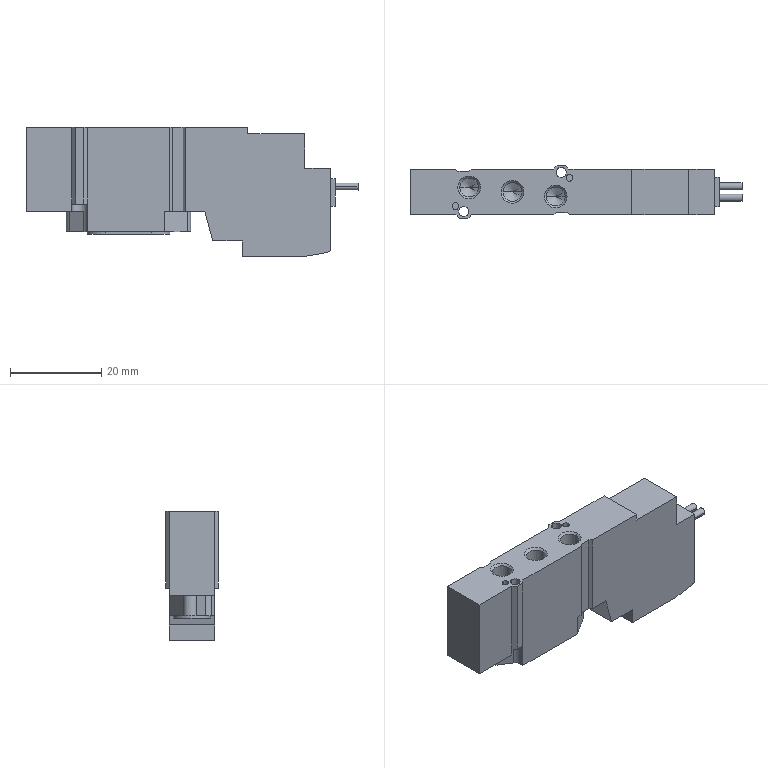Part | STEP file | 5-Port Solenoid Valve SY3120-5G-M5 | 1 solid | 120 faces | box 72.9 x 11.6 x 28.5 mm | volume 14643 mm3 | plane 56 | cylinder 36 | cone 28 | commonest cylinder face diameters 4.134 x10 1.5 x4 1.6 x4 2.2 x4 2.459 x4 3.4 x3